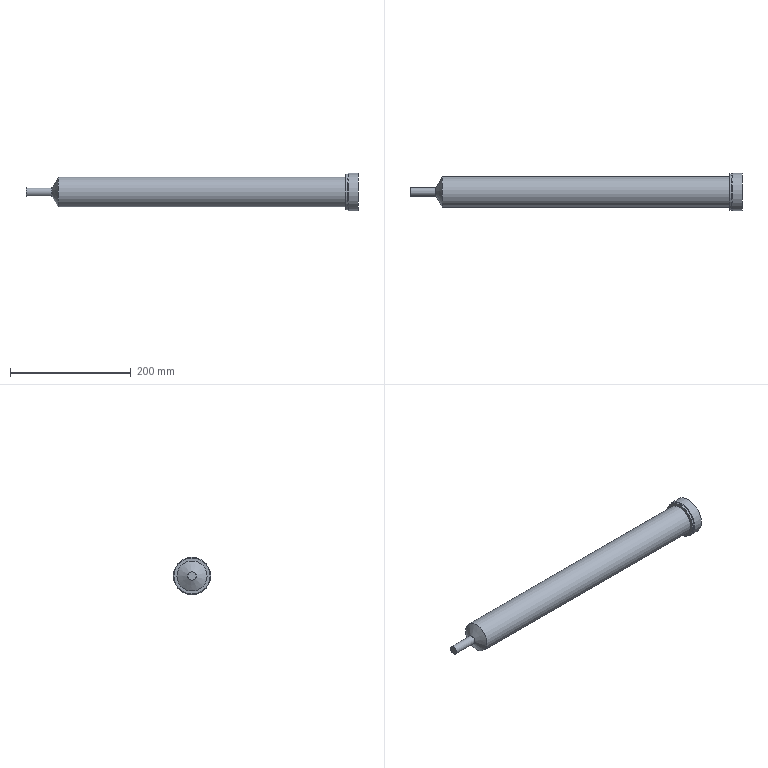Part | STEP file | 1 | 1 solid | 9 faces | box 550 x 62 x 62 mm | volume 1011386 mm3 | cylinder 4 | plane 3 | cone 2 | commonest cylinder face diameters 14 x1 50 x1 60 x1 62 x1